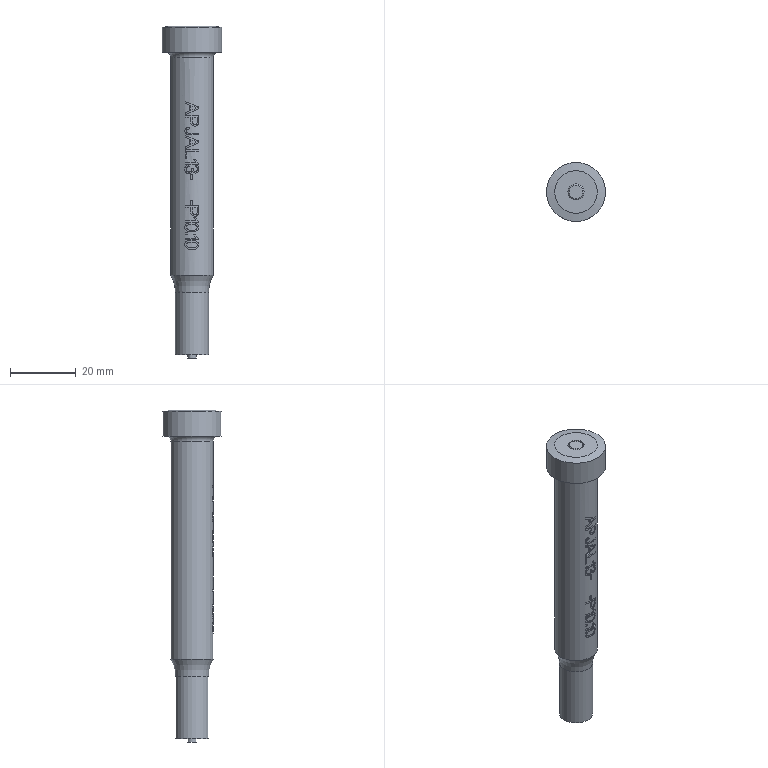Part | NX | features 8 2 | 1 solid | 175 faces | box 18 x 18 x 101 mm | volume 12938 mm3 | plane 105 | cylinder 65 | torus 2 | cone 2 | spline 1 | commonest cylinder face diameters 12.8 x15 13 x7 5.24 x3 5.884 x3 1.501 x2 1.782 x2